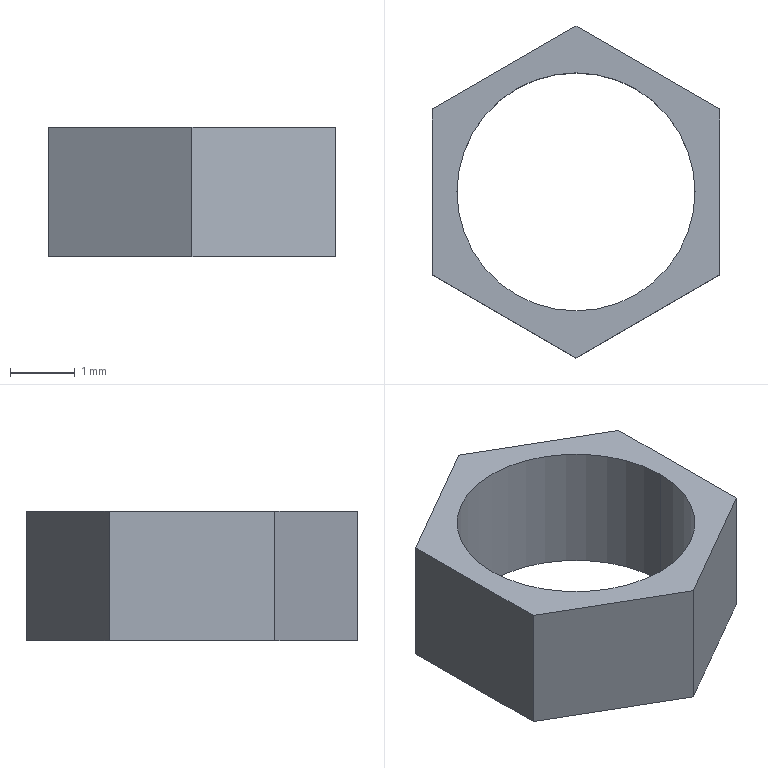Part | SolidWorks | features BaseBody 1 | 1 solid | 10 faces | box 4.422 x 5.106 x 2 mm | volume 12.787 mm3 | plane 8 | cylinder 2 | commonest cylinder face diameters 3.663 x2
STEP:
#1=CARTESIAN_POINT('',(4.678,-0.6848,0.));
#2=VERTEX_POINT('',#1);
#3=CARTESIAN_POINT('',(8.341,-0.6848,0.));
#4=VERTEX_POINT('',#3);
#5=CARTESIAN_POINT('',(6.51,-0.6848,0.));
#6=DIRECTION('',(0.,0.,1.));
#7=DIRECTION('',(1.,0.,0.));
#8=AXIS2_PLACEMENT_3D('',#5,#6,#7);
#9=CIRCLE('',#8,1.832);
#10=EDGE_CURVE('',#2,#4,#9,.T.);
#11=ORIENTED_EDGE('',*,*,#10,.F.);
#12=CARTESIAN_POINT('',(4.678,-0.6848,2.));
#13=VERTEX_POINT('',#12);
#14=CARTESIAN_POINT('',(4.678,-0.6848,0.));
#15=DIRECTION('',(0.,0.,1.));
#16=VECTOR('',#15,1000.);
#17=LINE('',#14,#16);
#18=EDGE_CURVE('',#2,#13,#17,.T.);
#19=ORIENTED_EDGE('',*,*,#18,.T.);
#20=CARTESIAN_POINT('',(8.341,-0.6848,2.));
#21=VERTEX_POINT('',#20);
#22=CARTESIAN_POINT('',(6.51,-0.6848,2.));
#23=DIRECTION('',(0.,0.,-1.));
#24=DIRECTION('',(1.,0.,0.));
#25=AXIS2_PLACEMENT_3D('',#22,#23,#24);
#26=CIRCLE('',#25,1.832);
#27=EDGE_CURVE('',#21,#13,#26,.T.);
#28=ORIENTED_EDGE('',*,*,#27,.F.);
#29=CARTESIAN_POINT('',(8.341,-0.6848,0.));
#30=DIRECTION('',(0.,0.,1.));
#31=VECTOR('',#30,1000.);
#32=LINE('',#29,#31);
#33=EDGE_CURVE('',#4,#21,#32,.T.);
#34=ORIENTED_EDGE('',*,*,#33,.F.);
#35=EDGE_LOOP('',(#11,#19,#28,#34));
#36=FACE_OUTER_BOUND('',#35,.T.);
#37=CARTESIAN_POINT('',(6.51,-0.6848,0.));
#38=DIRECTION('',(0.,0.,1.));
#39=DIRECTION('',(1.,0.,0.));
#40=AXIS2_PLACEMENT_3D('',#37,#38,#39);
#41=CYLINDRICAL_SURFACE('',#40,1.832);
#42=ADVANCED_FACE('',(#36),#41,.F.);
#43=ORIENTED_EDGE('',*,*,#18,.F.);
#44=CARTESIAN_POINT('',(6.51,-0.6848,0.));
#45=DIRECTION('',(0.,0.,1.));
#46=DIRECTION('',(1.,0.,0.));
#47=AXIS2_PLACEMENT_3D('',#44,#45,#46);
#48=CIRCLE('',#47,1.832);
#49=EDGE_CURVE('',#4,#2,#48,.T.);
#50=ORIENTED_EDGE('',*,*,#49,.F.);
#51=ORIENTED_EDGE('',*,*,#33,.T.);
#52=CARTESIAN_POINT('',(6.51,-0.6848,2.));
#53=DIRECTION('',(0.,0.,-1.));
#54=DIRECTION('',(1.,0.,0.));
#55=AXIS2_PLACEMENT_3D('',#52,#53,#54);
#56=CIRCLE('',#55,1.832);
#57=EDGE_CURVE('',#13,#21,#56,.T.);
#58=ORIENTED_EDGE('',*,*,#57,.F.);
#59=EDGE_LOOP('',(#43,#50,#51,#58));
#60=FACE_OUTER_BOUND('',#59,.T.);
#61=CARTESIAN_POINT('',(6.51,-0.6848,0.));
#62=DIRECTION('',(0.,0.,1.));
#63=DIRECTION('',(1.,0.,0.));
#64=AXIS2_PLACEMENT_3D('',#61,#62,#63);
#65=CYLINDRICAL_SURFACE('',#64,1.832);
#66=ADVANCED_FACE('',(#60),#65,.F.);
#67=ORIENTED_EDGE('',*,*,#27,.T.);
#68=ORIENTED_EDGE('',*,*,#57,.T.);
#69=EDGE_LOOP('',(#67,#68));
#70=FACE_BOUND('',#69,.T.);
#71=CARTESIAN_POINT('',(4.299,0.5917,2.));
#72=VERTEX_POINT('',#71);
#73=CARTESIAN_POINT('',(4.299,-1.961,2.));
#74=VERTEX_POINT('',#73);
#75=CARTESIAN_POINT('',(4.299,-0.6848,2.));
#76=DIRECTION('',(0.,-1.,0.));
#77=VECTOR('',#76,1000.);
#78=LINE('',#75,#77);
#79=EDGE_CURVE('',#72,#74,#78,.T.);
#80=ORIENTED_EDGE('',*,*,#79,.T.);
#81=CARTESIAN_POINT('',(6.51,-3.238,2.));
#82=VERTEX_POINT('',#81);
#83=CARTESIAN_POINT('',(4.299,-1.961,2.));
#84=DIRECTION('',(0.866,-0.5,0.));
#85=VECTOR('',#84,1000.);
#86=LINE('',#83,#85);
#87=EDGE_CURVE('',#74,#82,#86,.T.);
#88=ORIENTED_EDGE('',*,*,#87,.T.);
#89=CARTESIAN_POINT('',(8.721,-1.961,2.));
#90=VERTEX_POINT('',#89);
#91=CARTESIAN_POINT('',(6.51,-3.238,2.));
#92=DIRECTION('',(0.866,0.5,0.));
#93=VECTOR('',#92,1000.);
#94=LINE('',#91,#93);
#95=EDGE_CURVE('',#82,#90,#94,.T.);
#96=ORIENTED_EDGE('',*,*,#95,.T.);
#97=CARTESIAN_POINT('',(8.721,0.5917,2.));
#98=VERTEX_POINT('',#97);
#99=CARTESIAN_POINT('',(8.721,-0.6848,2.));
#100=DIRECTION('',(0.,1.,0.));
#101=VECTOR('',#100,1000.);
#102=LINE('',#99,#101);
#103=EDGE_CURVE('',#90,#98,#102,.T.);
#104=ORIENTED_EDGE('',*,*,#103,.T.);
#105=CARTESIAN_POINT('',(6.51,1.868,2.));
#106=VERTEX_POINT('',#105);
#107=CARTESIAN_POINT('',(8.721,0.5917,2.));
#108=DIRECTION('',(-0.866,0.5,0.));
#109=VECTOR('',#108,1000.);
#110=LINE('',#107,#109);
#111=EDGE_CURVE('',#98,#106,#110,.T.);
#112=ORIENTED_EDGE('',*,*,#111,.T.);
#113=CARTESIAN_POINT('',(6.51,1.868,2.));
#114=DIRECTION('',(-0.866,-0.5,0.));
#115=VECTOR('',#114,1000.);
#116=LINE('',#113,#115);
#117=EDGE_CURVE('',#106,#72,#116,.T.);
#118=ORIENTED_EDGE('',*,*,#117,.T.);
#119=EDGE_LOOP('',(#80,#88,#96,#104,#112,#118));
#120=FACE_OUTER_BOUND('',#119,.T.);
#121=CARTESIAN_POINT('',(6.51,-0.6848,2.));
#122=DIRECTION('',(0.,0.,1.));
#123=DIRECTION('',(1.,0.,0.));
#124=AXIS2_PLACEMENT_3D('',#121,#122,#123);
#125=PLANE('',#124);
#126=ADVANCED_FACE('',(#70,#120),#125,.T.);
#127=ORIENTED_EDGE('',*,*,#49,.T.);
#128=ORIENTED_EDGE('',*,*,#10,.T.);
#129=EDGE_LOOP('',(#127,#128));
#130=FACE_BOUND('',#129,.T.);
#131=CARTESIAN_POINT('',(4.299,-1.961,0.));
#132=VERTEX_POINT('',#131);
#133=CARTESIAN_POINT('',(6.51,-3.238,0.));
#134=VERTEX_POINT('',#133);
#135=CARTESIAN_POINT('',(4.299,-1.961,0.));
#136=DIRECTION('',(0.866,-0.5,0.));
#137=VECTOR('',#136,1000.);
#138=LINE('',#135,#137);
#139=EDGE_CURVE('',#132,#134,#138,.T.);
#140=ORIENTED_EDGE('',*,*,#139,.F.);
#141=CARTESIAN_POINT('',(4.299,0.5917,0.));
#142=VERTEX_POINT('',#141);
#143=CARTESIAN_POINT('',(4.299,-0.6848,0.));
#144=DIRECTION('',(0.,-1.,0.));
#145=VECTOR('',#144,1000.);
#146=LINE('',#143,#145);
#147=EDGE_CURVE('',#142,#132,#146,.T.);
#148=ORIENTED_EDGE('',*,*,#147,.F.);
#149=CARTESIAN_POINT('',(6.51,1.868,0.));
#150=VERTEX_POINT('',#149);
#151=CARTESIAN_POINT('',(6.51,1.868,0.));
#152=DIRECTION('',(-0.866,-0.5,0.));
#153=VECTOR('',#152,1000.);
#154=LINE('',#151,#153);
#155=EDGE_CURVE('',#150,#142,#154,.T.);
#156=ORIENTED_EDGE('',*,*,#155,.F.);
#157=CARTESIAN_POINT('',(8.721,0.5917,0.));
#158=VERTEX_POINT('',#157);
#159=CARTESIAN_POINT('',(8.721,0.5917,0.));
#160=DIRECTION('',(-0.866,0.5,0.));
#161=VECTOR('',#160,1000.);
#162=LINE('',#159,#161);
#163=EDGE_CURVE('',#158,#150,#162,.T.);
#164=ORIENTED_EDGE('',*,*,#163,.F.);
#165=CARTESIAN_POINT('',(8.721,-1.961,0.));
#166=VERTEX_POINT('',#165);
#167=CARTESIAN_POINT('',(8.721,-0.6848,0.));
#168=DIRECTION('',(0.,1.,0.));
#169=VECTOR('',#168,1000.);
#170=LINE('',#167,#169);
#171=EDGE_CURVE('',#166,#158,#170,.T.);
#172=ORIENTED_EDGE('',*,*,#171,.F.);
#173=CARTESIAN_POINT('',(6.51,-3.238,0.));
#174=DIRECTION('',(0.866,0.5,0.));
#175=VECTOR('',#174,1000.);
#176=LINE('',#173,#175);
#177=EDGE_CURVE('',#134,#166,#176,.T.);
#178=ORIENTED_EDGE('',*,*,#177,.F.);
#179=EDGE_LOOP('',(#140,#148,#156,#164,#172,#178));
#180=FACE_OUTER_BOUND('',#179,.T.);
#181=CARTESIAN_POINT('',(6.51,-0.6848,0.));
#182=DIRECTION('',(0.,0.,1.));
#183=DIRECTION('',(1.,0.,0.));
#184=AXIS2_PLACEMENT_3D('',#181,#182,#183);
#185=PLANE('',#184);
#186=ADVANCED_FACE('',(#130,#180),#185,.F.);
#187=ORIENTED_EDGE('',*,*,#87,.F.);
#188=CARTESIAN_POINT('',(4.299,-1.961,0.));
#189=DIRECTION('',(0.,0.,-1.));
#190=VECTOR('',#189,1000.);
#191=LINE('',#188,#190);
#192=EDGE_CURVE('',#74,#132,#191,.T.);
#193=ORIENTED_EDGE('',*,*,#192,.T.);
#194=ORIENTED_EDGE('',*,*,#139,.T.);
#195=CARTESIAN_POINT('',(6.51,-3.238,0.));
#196=DIRECTION('',(0.,0.,1.));
#197=VECTOR('',#196,1000.);
#198=LINE('',#195,#197);
#199=EDGE_CURVE('',#134,#82,#198,.T.);
#200=ORIENTED_EDGE('',*,*,#199,.T.);
#201=EDGE_LOOP('',(#187,#193,#194,#200));
#202=FACE_OUTER_BOUND('',#201,.T.);
#203=CARTESIAN_POINT('',(4.299,-1.961,0.));
#204=DIRECTION('',(-0.5,-0.866,0.));
#205=DIRECTION('',(0.866,-0.5,0.));
#206=AXIS2_PLACEMENT_3D('',#203,#204,#205);
#207=PLANE('',#206);
#208=ADVANCED_FACE('',(#202),#207,.T.);
#209=ORIENTED_EDGE('',*,*,#79,.F.);
#210=CARTESIAN_POINT('',(4.299,0.5917,0.));
#211=DIRECTION('',(0.,0.,-1.));
#212=VECTOR('',#211,1000.);
#213=LINE('',#210,#212);
#214=EDGE_CURVE('',#72,#142,#213,.T.);
#215=ORIENTED_EDGE('',*,*,#214,.T.);
#216=ORIENTED_EDGE('',*,*,#147,.T.);
#217=ORIENTED_EDGE('',*,*,#192,.F.);
#218=EDGE_LOOP('',(#209,#215,#216,#217));
#219=FACE_OUTER_BOUND('',#218,.T.);
#220=CARTESIAN_POINT('',(4.299,0.5917,0.));
#221=DIRECTION('',(-1.,0.,0.));
#222=DIRECTION('',(0.,-1.,0.));
#223=AXIS2_PLACEMENT_3D('',#220,#221,#222);
#224=PLANE('',#223);
#225=ADVANCED_FACE('',(#219),#224,.T.);
#226=ORIENTED_EDGE('',*,*,#117,.F.);
#227=CARTESIAN_POINT('',(6.51,1.868,0.));
#228=DIRECTION('',(0.,0.,-1.));
#229=VECTOR('',#228,1000.);
#230=LINE('',#227,#229);
#231=EDGE_CURVE('',#106,#150,#230,.T.);
#232=ORIENTED_EDGE('',*,*,#231,.T.);
#233=ORIENTED_EDGE('',*,*,#155,.T.);
#234=ORIENTED_EDGE('',*,*,#214,.F.);
#235=EDGE_LOOP('',(#226,#232,#233,#234));
#236=FACE_OUTER_BOUND('',#235,.T.);
#237=CARTESIAN_POINT('',(6.51,1.868,0.));
#238=DIRECTION('',(-0.5,0.866,0.));
#239=DIRECTION('',(-0.866,-0.5,0.));
#240=AXIS2_PLACEMENT_3D('',#237,#238,#239);
#241=PLANE('',#240);
#242=ADVANCED_FACE('',(#236),#241,.T.);
#243=ORIENTED_EDGE('',*,*,#111,.F.);
#244=CARTESIAN_POINT('',(8.721,0.5917,0.));
#245=DIRECTION('',(0.,0.,-1.));
#246=VECTOR('',#245,1000.);
#247=LINE('',#244,#246);
#248=EDGE_CURVE('',#98,#158,#247,.T.);
#249=ORIENTED_EDGE('',*,*,#248,.T.);
#250=ORIENTED_EDGE('',*,*,#163,.T.);
#251=ORIENTED_EDGE('',*,*,#231,.F.);
#252=EDGE_LOOP('',(#243,#249,#250,#251));
#253=FACE_OUTER_BOUND('',#252,.T.);
#254=CARTESIAN_POINT('',(8.721,0.5917,0.));
#255=DIRECTION('',(0.5,0.866,0.));
#256=DIRECTION('',(-0.866,0.5,0.));
#257=AXIS2_PLACEMENT_3D('',#254,#255,#256);
#258=PLANE('',#257);
#259=ADVANCED_FACE('',(#253),#258,.T.);
#260=ORIENTED_EDGE('',*,*,#103,.F.);
#261=CARTESIAN_POINT('',(8.721,-1.961,0.));
#262=DIRECTION('',(0.,0.,-1.));
#263=VECTOR('',#262,1000.);
#264=LINE('',#261,#263);
#265=EDGE_CURVE('',#90,#166,#264,.T.);
#266=ORIENTED_EDGE('',*,*,#265,.T.);
#267=ORIENTED_EDGE('',*,*,#171,.T.);
#268=ORIENTED_EDGE('',*,*,#248,.F.);
#269=EDGE_LOOP('',(#260,#266,#267,#268));
#270=FACE_OUTER_BOUND('',#269,.T.);
#271=CARTESIAN_POINT('',(8.721,-1.961,0.));
#272=DIRECTION('',(1.,0.,0.));
#273=DIRECTION('',(0.,0.,-1.));
#274=AXIS2_PLACEMENT_3D('',#271,#272,#273);
#275=PLANE('',#274);
#276=ADVANCED_FACE('',(#270),#275,.T.);
#277=ORIENTED_EDGE('',*,*,#95,.F.);
#278=ORIENTED_EDGE('',*,*,#199,.F.);
#279=ORIENTED_EDGE('',*,*,#177,.T.);
#280=ORIENTED_EDGE('',*,*,#265,.F.);
#281=EDGE_LOOP('',(#277,#278,#279,#280));
#282=FACE_OUTER_BOUND('',#281,.T.);
#283=CARTESIAN_POINT('',(6.51,-3.238,0.));
#284=DIRECTION('',(0.5,-0.866,0.));
#285=DIRECTION('',(0.866,0.5,0.));
#286=AXIS2_PLACEMENT_3D('',#283,#284,#285);
#287=PLANE('',#286);
#288=ADVANCED_FACE('',(#282),#287,.T.);
#289=CLOSED_SHELL('',(#42,#66,#126,#186,#208,#225,#242,#259,#276,#288));
#290=MANIFOLD_SOLID_BREP('',#289);
#291=CARTESIAN_POINT('',(0.,0.,0.));
#292=DIRECTION('',(0.,0.,1.));
#293=DIRECTION('',(1.,0.,0.));
#294=AXIS2_PLACEMENT_3D('',#291,#292,#293);
#295=(LENGTH_UNIT()NAMED_UNIT(*)SI_UNIT(.MILLI.,.METRE.));
#296=UNCERTAINTY_MEASURE_WITH_UNIT(LENGTH_MEASURE(0.00001),#295,'','');
#297=(NAMED_UNIT(*)PLANE_ANGLE_UNIT()SI_UNIT($,.RADIAN.));
#298=(NAMED_UNIT(*)SI_UNIT($,.STERADIAN.)SOLID_ANGLE_UNIT());
#299=(GEOMETRIC_REPRESENTATION_CONTEXT(3)GLOBAL_UNCERTAINTY_ASSIGNED_CONTEXT((#296))GLOBAL_UNIT_ASSIGNED_CONTEXT((#295,#297,#298))REPRESENTATION_CONTEXT('',''));
#300=ADVANCED_BREP_SHAPE_REPRESENTATION('',(#290,#294),#299);